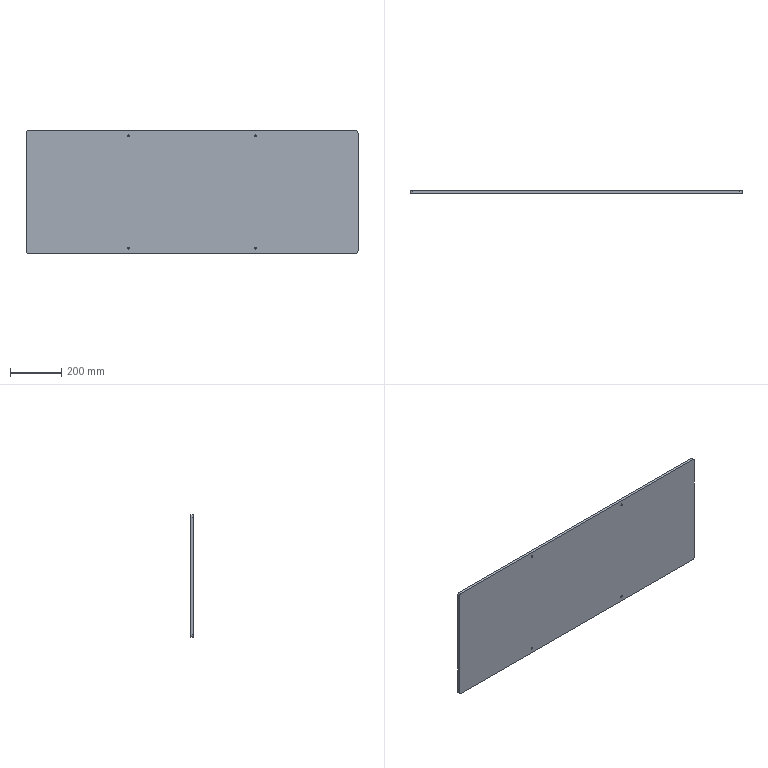Part | STEP file | H_ND24021-01-JG-103-TL | 1 solid | 30 faces | box 1300 x 10 x 480 mm | volume 6236216 mm3 | cylinder 20 | plane 10 | commonest cylinder face diameters 6.6 x8 11 x8 20 x4